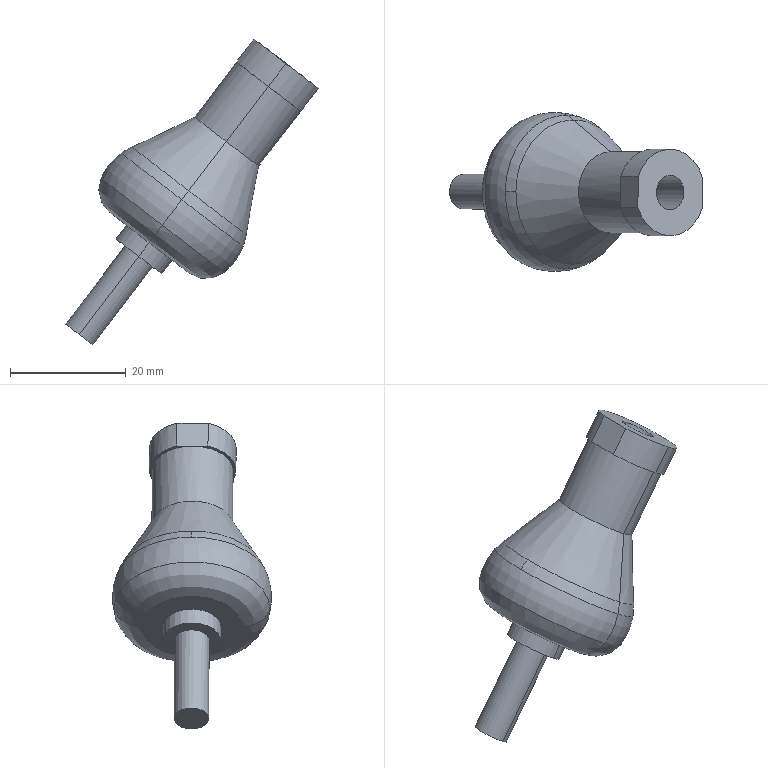Part | STEP file | 46B-01003ZX30 | 1 solid | 31 faces | box 43.778 x 27.592 x 52.956 mm | volume 12356 mm3 | cylinder 12 | plane 9 | torus 4 | sphere 4 | cone 2 | commonest cylinder face diameters 6 x4 15 x4 10 x2 14 x2
STEP:
#1=CARTESIAN_POINT('',(34.169,-36.791,43.691));
#2=VERTEX_POINT('',#1);
#3=CARTESIAN_POINT('',(34.207,-30.791,43.691));
#4=VERTEX_POINT('',#3);
#5=CARTESIAN_POINT('',(34.188,-33.791,43.691));
#6=DIRECTION('',(0.607,-0.003842,0.7947));
#7=AXIS2_PLACEMENT_3D('',#5,#6,$);
#8=CIRCLE('',#7,3.);
#9=EDGE_CURVE('',#2,#4,#8,.F.);
#10=ORIENTED_EDGE('',*,*,#9,.F.);
#11=CARTESIAN_POINT('',(44.488,-36.856,57.2));
#12=VERTEX_POINT('',#11);
#13=CARTESIAN_POINT('',(34.169,-36.791,43.691));
#14=DIRECTION('',(0.607,-0.003842,0.7947));
#15=VECTOR('',#14,1.);
#16=LINE('',#13,#15);
#17=EDGE_CURVE('',#2,#12,#16,.T.);
#18=ORIENTED_EDGE('',*,*,#17,.T.);
#19=CARTESIAN_POINT('',(44.526,-30.856,57.2));
#20=VERTEX_POINT('',#19);
#21=CARTESIAN_POINT('',(44.507,-33.856,57.2));
#22=DIRECTION('',(0.607,-0.003842,0.7947));
#23=AXIS2_PLACEMENT_3D('',#21,#22,$);
#24=CIRCLE('',#23,3.);
#25=EDGE_CURVE('',#12,#20,#24,.F.);
#26=ORIENTED_EDGE('',*,*,#25,.T.);
#27=CARTESIAN_POINT('',(34.207,-30.791,43.691));
#28=DIRECTION('',(0.607,-0.003842,0.7947));
#29=VECTOR('',#28,1.);
#30=LINE('',#27,#29);
#31=EDGE_CURVE('',#4,#20,#30,.T.);
#32=ORIENTED_EDGE('',*,*,#31,.F.);
#33=EDGE_LOOP('',(#10,#18,#26,#32));
#34=FACE_OUTER_BOUND('',#33,.T.);
#35=CARTESIAN_POINT('',(34.188,-33.791,43.691));
#36=DIRECTION('',(0.607,-0.003842,0.7947));
#37=DIRECTION('',(0.006329,1.,0.));
#38=AXIS2_PLACEMENT_3D('',#35,#36,#37);
#39=CYLINDRICAL_SURFACE('',#38,3.);
#40=ADVANCED_FACE('',(#34),#39,.T.);
#41=CARTESIAN_POINT('',(34.188,-33.791,43.691));
#42=DIRECTION('',(-0.607,0.003842,-0.7947));
#43=AXIS2_PLACEMENT_3D('',#41,#42,$);
#44=CIRCLE('',#43,3.);
#45=EDGE_CURVE('',#4,#2,#44,.T.);
#46=ORIENTED_EDGE('',*,*,#45,.T.);
#47=ORIENTED_EDGE('',*,*,#9,.T.);
#48=EDGE_LOOP('',(#46,#47));
#49=FACE_OUTER_BOUND('',#48,.T.);
#50=CARTESIAN_POINT('',(34.188,-33.791,43.691));
#51=DIRECTION('',(-0.607,0.003842,-0.7947));
#52=DIRECTION('',(-0.006329,-1.,0.));
#53=AXIS2_PLACEMENT_3D('',#50,#51,#52);
#54=PLANE('',#53);
#55=ADVANCED_FACE('',(#49),#54,.T.);
#56=ORIENTED_EDGE('',*,*,#17,.F.);
#57=ORIENTED_EDGE('',*,*,#45,.F.);
#58=ORIENTED_EDGE('',*,*,#31,.T.);
#59=CARTESIAN_POINT('',(44.507,-33.856,57.2));
#60=DIRECTION('',(0.607,-0.003842,0.7947));
#61=AXIS2_PLACEMENT_3D('',#59,#60,$);
#62=CIRCLE('',#61,3.);
#63=EDGE_CURVE('',#20,#12,#62,.F.);
#64=ORIENTED_EDGE('',*,*,#63,.T.);
#65=EDGE_LOOP('',(#56,#57,#58,#64));
#66=FACE_OUTER_BOUND('',#65,.T.);
#67=CARTESIAN_POINT('',(34.188,-33.791,43.691));
#68=DIRECTION('',(0.607,-0.003842,0.7947));
#69=DIRECTION('',(-0.006329,-1.,0.));
#70=AXIS2_PLACEMENT_3D('',#67,#68,#69);
#71=CYLINDRICAL_SURFACE('',#70,3.);
#72=ADVANCED_FACE('',(#66),#71,.T.);
#73=CARTESIAN_POINT('',(44.539,-28.857,57.2));
#74=VERTEX_POINT('',#73);
#75=CARTESIAN_POINT('',(44.476,-38.856,57.2));
#76=VERTEX_POINT('',#75);
#77=CARTESIAN_POINT('',(44.507,-33.856,57.2));
#78=DIRECTION('',(-0.607,0.003842,-0.7947));
#79=AXIS2_PLACEMENT_3D('',#77,#78,$);
#80=CIRCLE('',#79,5.);
#81=EDGE_CURVE('',#74,#76,#80,.T.);
#82=ORIENTED_EDGE('',*,*,#81,.T.);
#83=CARTESIAN_POINT('',(44.507,-33.856,57.2));
#84=DIRECTION('',(-0.607,0.003842,-0.7947));
#85=AXIS2_PLACEMENT_3D('',#83,#84,$);
#86=CIRCLE('',#85,5.);
#87=EDGE_CURVE('',#76,#74,#86,.T.);
#88=ORIENTED_EDGE('',*,*,#87,.T.);
#89=EDGE_LOOP('',(#82,#88));
#90=FACE_OUTER_BOUND('',#89,.T.);
#91=ORIENTED_EDGE('',*,*,#63,.F.);
#92=ORIENTED_EDGE('',*,*,#25,.F.);
#93=EDGE_LOOP('',(#91,#92));
#94=FACE_BOUND('',#93,.T.);
#95=CARTESIAN_POINT('',(44.507,-33.856,57.2));
#96=DIRECTION('',(-0.607,0.003842,-0.7947));
#97=DIRECTION('',(-0.006329,-1.,0.));
#98=AXIS2_PLACEMENT_3D('',#95,#96,#97);
#99=PLANE('',#98);
#100=ADVANCED_FACE('',(#90,#94),#99,.T.);
#101=CARTESIAN_POINT('',(46.297,-38.868,59.584));
#102=VERTEX_POINT('',#101);
#103=CARTESIAN_POINT('',(44.476,-38.856,57.2));
#104=DIRECTION('',(0.607,-0.003842,0.7947));
#105=VECTOR('',#104,1.);
#106=LINE('',#103,#105);
#107=EDGE_CURVE('',#76,#102,#106,.T.);
#108=ORIENTED_EDGE('',*,*,#107,.F.);
#109=ORIENTED_EDGE('',*,*,#81,.F.);
#110=CARTESIAN_POINT('',(46.36,-28.868,59.584));
#111=VERTEX_POINT('',#110);
#112=CARTESIAN_POINT('',(44.539,-28.857,57.2));
#113=DIRECTION('',(0.607,-0.003842,0.7947));
#114=VECTOR('',#113,1.);
#115=LINE('',#112,#114);
#116=EDGE_CURVE('',#74,#111,#115,.T.);
#117=ORIENTED_EDGE('',*,*,#116,.T.);
#118=CARTESIAN_POINT('',(46.328,-33.868,59.584));
#119=DIRECTION('',(0.607,-0.003842,0.7947));
#120=AXIS2_PLACEMENT_3D('',#118,#119,$);
#121=CIRCLE('',#120,5.);
#122=EDGE_CURVE('',#111,#102,#121,.F.);
#123=ORIENTED_EDGE('',*,*,#122,.T.);
#124=EDGE_LOOP('',(#108,#109,#117,#123));
#125=FACE_OUTER_BOUND('',#124,.T.);
#126=CARTESIAN_POINT('',(44.507,-33.856,57.2));
#127=DIRECTION('',(0.607,-0.003842,0.7947));
#128=DIRECTION('',(-0.006329,-1.,0.));
#129=AXIS2_PLACEMENT_3D('',#126,#127,#128);
#130=CYLINDRICAL_SURFACE('',#129,5.);
#131=ADVANCED_FACE('',(#125),#130,.T.);
#132=ORIENTED_EDGE('',*,*,#87,.F.);
#133=ORIENTED_EDGE('',*,*,#107,.T.);
#134=CARTESIAN_POINT('',(46.328,-33.868,59.584));
#135=DIRECTION('',(0.607,-0.003842,0.7947));
#136=AXIS2_PLACEMENT_3D('',#134,#135,$);
#137=CIRCLE('',#136,5.);
#138=EDGE_CURVE('',#102,#111,#137,.F.);
#139=ORIENTED_EDGE('',*,*,#138,.T.);
#140=ORIENTED_EDGE('',*,*,#116,.F.);
#141=EDGE_LOOP('',(#132,#133,#139,#140));
#142=FACE_OUTER_BOUND('',#141,.T.);
#143=CARTESIAN_POINT('',(44.507,-33.856,57.2));
#144=DIRECTION('',(0.607,-0.003842,0.7947));
#145=DIRECTION('',(0.006329,1.,0.));
#146=AXIS2_PLACEMENT_3D('',#143,#144,#145);
#147=CYLINDRICAL_SURFACE('',#146,5.);
#148=ADVANCED_FACE('',(#142),#147,.T.);
#149=CARTESIAN_POINT('',(46.274,-42.517,59.584));
#150=VERTEX_POINT('',#149);
#151=CARTESIAN_POINT('',(46.383,-25.219,59.584));
#152=VERTEX_POINT('',#151);
#153=CARTESIAN_POINT('',(46.328,-33.868,59.584));
#154=DIRECTION('',(-0.607,0.003842,-0.7947));
#155=AXIS2_PLACEMENT_3D('',#153,#154,$);
#156=CIRCLE('',#155,8.649);
#157=EDGE_CURVE('',#150,#152,#156,.T.);
#158=ORIENTED_EDGE('',*,*,#157,.T.);
#159=CARTESIAN_POINT('',(46.328,-33.868,59.584));
#160=DIRECTION('',(-0.607,0.003842,-0.7947));
#161=AXIS2_PLACEMENT_3D('',#159,#160,$);
#162=CIRCLE('',#161,8.649);
#163=EDGE_CURVE('',#152,#150,#162,.T.);
#164=ORIENTED_EDGE('',*,*,#163,.T.);
#165=EDGE_LOOP('',(#158,#164));
#166=FACE_OUTER_BOUND('',#165,.T.);
#167=ORIENTED_EDGE('',*,*,#122,.F.);
#168=ORIENTED_EDGE('',*,*,#138,.F.);
#169=EDGE_LOOP('',(#167,#168));
#170=FACE_BOUND('',#169,.T.);
#171=CARTESIAN_POINT('',(46.328,-33.868,59.584));
#172=DIRECTION('',(-0.607,0.003842,-0.7947));
#173=DIRECTION('',(-0.006329,-1.,0.));
#174=AXIS2_PLACEMENT_3D('',#171,#172,#173);
#175=PLANE('',#174);
#176=ADVANCED_FACE('',(#166,#170),#175,.T.);
#177=CARTESIAN_POINT('',(48.719,-20.38,62.602));
#178=VERTEX_POINT('',#177);
#179=CARTESIAN_POINT('',(48.548,-47.385,62.602));
#180=VERTEX_POINT('',#179);
#181=CARTESIAN_POINT('',(48.633,-33.883,62.602));
#182=DIRECTION('',(-0.607,0.003842,-0.7947));
#183=AXIS2_PLACEMENT_3D('',#181,#182,$);
#184=CIRCLE('',#183,13.502);
#185=EDGE_CURVE('',#178,#180,#184,.F.);
#186=ORIENTED_EDGE('',*,*,#185,.F.);
#187=CARTESIAN_POINT('',(49.418,-25.238,63.558));
#188=DIRECTION('',(-0.7947,0.00503,0.607));
#189=AXIS2_PLACEMENT_3D('',#187,#188,$);
#190=CIRCLE('',#189,5.);
#191=EDGE_CURVE('',#178,#152,#190,.T.);
#192=ORIENTED_EDGE('',*,*,#191,.T.);
#193=ORIENTED_EDGE('',*,*,#157,.F.);
#194=CARTESIAN_POINT('',(49.309,-42.536,63.558));
#195=DIRECTION('',(0.7947,-0.00503,-0.607));
#196=AXIS2_PLACEMENT_3D('',#194,#195,$);
#197=CIRCLE('',#196,5.);
#198=EDGE_CURVE('',#180,#150,#197,.T.);
#199=ORIENTED_EDGE('',*,*,#198,.F.);
#200=EDGE_LOOP('',(#186,#192,#193,#199));
#201=FACE_OUTER_BOUND('',#200,.T.);
#202=CARTESIAN_POINT('',(49.364,-33.887,63.558));
#203=DIRECTION('',(-0.607,0.003842,-0.7947));
#204=DIRECTION('',(-0.006329,-1.,0.));
#205=AXIS2_PLACEMENT_3D('',#202,#203,#204);
#206=TOROIDAL_SURFACE('',#205,8.649,5.);
#207=ADVANCED_FACE('',(#201),#206,.T.);
#208=ORIENTED_EDGE('',*,*,#191,.F.);
#209=CARTESIAN_POINT('',(48.633,-33.883,62.602));
#210=DIRECTION('',(-0.607,0.003842,-0.7947));
#211=AXIS2_PLACEMENT_3D('',#209,#210,$);
#212=CIRCLE('',#211,13.502);
#213=EDGE_CURVE('',#180,#178,#212,.F.);
#214=ORIENTED_EDGE('',*,*,#213,.F.);
#215=ORIENTED_EDGE('',*,*,#198,.T.);
#216=ORIENTED_EDGE('',*,*,#163,.F.);
#217=EDGE_LOOP('',(#208,#214,#215,#216));
#218=FACE_OUTER_BOUND('',#217,.T.);
#219=CARTESIAN_POINT('',(49.364,-33.887,63.558));
#220=DIRECTION('',(-0.607,0.003842,-0.7947));
#221=DIRECTION('',(0.006329,1.,0.));
#222=AXIS2_PLACEMENT_3D('',#219,#220,#221);
#223=TOROIDAL_SURFACE('',#222,8.649,5.);
#224=ADVANCED_FACE('',(#218),#223,.T.);
#225=CARTESIAN_POINT('',(52.092,-20.618,67.019));
#226=VERTEX_POINT('',#225);
#227=CARTESIAN_POINT('',(41.45,-33.837,75.084));
#228=VERTEX_POINT('',#227);
#229=CARTESIAN_POINT('',(52.008,-33.904,67.019));
#230=DIRECTION('',(-0.607,0.003842,-0.7947));
#231=AXIS2_PLACEMENT_3D('',#229,#230,$);
#232=CIRCLE('',#231,13.286);
#233=EDGE_CURVE('',#226,#228,#232,.F.);
#234=ORIENTED_EDGE('',*,*,#233,.F.);
#235=CARTESIAN_POINT('',(50.118,-30.096,64.513));
#236=DIRECTION('',(-0.7947,0.00503,0.607));
#237=AXIS2_PLACEMENT_3D('',#235,#236,$);
#238=CIRCLE('',#237,10.);
#239=EDGE_CURVE('',#226,#178,#238,.T.);
#240=ORIENTED_EDGE('',*,*,#239,.T.);
#241=ORIENTED_EDGE('',*,*,#185,.T.);
#242=CARTESIAN_POINT('',(51.924,-47.189,67.019));
#243=VERTEX_POINT('',#242);
#244=CARTESIAN_POINT('',(50.069,-37.688,64.513));
#245=DIRECTION('',(0.7947,-0.00503,-0.607));
#246=AXIS2_PLACEMENT_3D('',#244,#245,$);
#247=CIRCLE('',#246,10.);
#248=EDGE_CURVE('',#243,#180,#247,.T.);
#249=ORIENTED_EDGE('',*,*,#248,.F.);
#250=CARTESIAN_POINT('',(52.008,-33.904,67.019));
#251=DIRECTION('',(-0.607,0.003842,-0.7947));
#252=AXIS2_PLACEMENT_3D('',#250,#251,$);
#253=CIRCLE('',#252,13.286);
#254=EDGE_CURVE('',#228,#243,#253,.F.);
#255=ORIENTED_EDGE('',*,*,#254,.F.);
#256=EDGE_LOOP('',(#234,#240,#241,#249,#255));
#257=FACE_OUTER_BOUND('',#256,.T.);
#258=CARTESIAN_POINT('',(50.094,-33.892,64.513));
#259=DIRECTION('',(-0.607,0.003842,-0.7947));
#260=DIRECTION('',(-0.006329,-1.,0.));
#261=AXIS2_PLACEMENT_3D('',#258,#259,#260);
#262=DEGENERATE_TOROIDAL_SURFACE('',#261,3.796,10.,.T.);
#263=ADVANCED_FACE('',(#257),#262,.T.);
#264=ORIENTED_EDGE('',*,*,#239,.F.);
#265=CARTESIAN_POINT('',(62.565,-33.971,58.954));
#266=VERTEX_POINT('',#265);
#267=CARTESIAN_POINT('',(52.008,-33.904,67.019));
#268=DIRECTION('',(-0.607,0.003842,-0.7947));
#269=AXIS2_PLACEMENT_3D('',#267,#268,$);
#270=CIRCLE('',#269,13.286);
#271=EDGE_CURVE('',#266,#226,#270,.F.);
#272=ORIENTED_EDGE('',*,*,#271,.F.);
#273=CARTESIAN_POINT('',(52.008,-33.904,67.019));
#274=DIRECTION('',(-0.607,0.003842,-0.7947));
#275=AXIS2_PLACEMENT_3D('',#273,#274,$);
#276=CIRCLE('',#275,13.286);
#277=EDGE_CURVE('',#243,#266,#276,.F.);
#278=ORIENTED_EDGE('',*,*,#277,.F.);
#279=ORIENTED_EDGE('',*,*,#248,.T.);
#280=ORIENTED_EDGE('',*,*,#213,.T.);
#281=EDGE_LOOP('',(#264,#272,#278,#279,#280));
#282=FACE_OUTER_BOUND('',#281,.T.);
#283=CARTESIAN_POINT('',(50.094,-33.892,64.513));
#284=DIRECTION('',(-0.607,0.003842,-0.7947));
#285=DIRECTION('',(0.006329,1.,0.));
#286=AXIS2_PLACEMENT_3D('',#283,#284,#285);
#287=DEGENERATE_TOROIDAL_SURFACE('',#286,3.796,10.,.T.);
#288=ADVANCED_FACE('',(#282),#287,.T.);
#289=CARTESIAN_POINT('',(53.277,-21.447,68.577));
#290=VERTEX_POINT('',#289);
#291=CARTESIAN_POINT('',(49.328,-33.887,63.511));
#292=DIRECTION('',(0.7947,-0.00503,-0.607));
#293=AXIS2_PLACEMENT_3D('',#291,#292,$);
#294=CIRCLE('',#293,14.);
#295=EDGE_CURVE('',#226,#290,#294,.T.);
#296=ORIENTED_EDGE('',*,*,#295,.F.);
#297=ORIENTED_EDGE('',*,*,#233,.T.);
#298=CARTESIAN_POINT('',(43.293,-33.849,76.143));
#299=VERTEX_POINT('',#298);
#300=CARTESIAN_POINT('',(49.328,-33.887,63.511));
#301=DIRECTION('',(-0.006329,-1.,0.));
#302=AXIS2_PLACEMENT_3D('',#300,#301,$);
#303=CIRCLE('',#302,14.);
#304=EDGE_CURVE('',#228,#299,#303,.F.);
#305=ORIENTED_EDGE('',*,*,#304,.T.);
#306=CARTESIAN_POINT('',(53.277,-21.447,68.577));
#307=CARTESIAN_POINT('',(52.881,-21.445,68.879));
#308=CARTESIAN_POINT('',(52.485,-21.467,69.181));
#309=CARTESIAN_POINT('',(52.082,-21.514,69.489));
#310=CARTESIAN_POINT('',(51.216,-21.672,70.15));
#311=CARTESIAN_POINT('',(50.266,-21.99,70.874));
#312=CARTESIAN_POINT('',(49.746,-22.207,71.27));
#313=CARTESIAN_POINT('',(48.645,-22.788,72.108));
#314=CARTESIAN_POINT('',(47.509,-23.675,72.972));
#315=CARTESIAN_POINT('',(46.946,-24.205,73.399));
#316=CARTESIAN_POINT('',(45.885,-25.41,74.204));
#317=CARTESIAN_POINT('',(44.991,-26.871,74.88));
#318=CARTESIAN_POINT('',(44.598,-27.656,75.176));
#319=CARTESIAN_POINT('',(43.93,-29.311,75.679));
#320=CARTESIAN_POINT('',(43.513,-31.094,75.988));
#321=CARTESIAN_POINT('',(43.372,-32.005,76.091));
#322=CARTESIAN_POINT('',(43.299,-32.927,76.143));
#323=CARTESIAN_POINT('',(43.293,-33.849,76.143));
#324=B_SPLINE_CURVE_WITH_KNOTS('',5,(#306,#307,#308,#309,#310,#311,#312,#313,#314,#315,#316,#317,#318,#319,#320,#321,#322,#323),.UNSPECIFIED.,.F.,.U.,(6,3,3,3,3,6),(0.,6.005,12.466,19.014,25.534,32.054),.UNSPECIFIED.);
#325=EDGE_CURVE('',#290,#299,#324,.T.);
#326=ORIENTED_EDGE('',*,*,#325,.F.);
#327=EDGE_LOOP('',(#296,#297,#305,#326));
#328=FACE_OUTER_BOUND('',#327,.T.);
#329=CARTESIAN_POINT('',(49.328,-33.887,63.511));
#330=DIRECTION('',(-0.006329,-1.,0.));
#331=DIRECTION('',(0.607,-0.003842,0.7947));
#332=AXIS2_PLACEMENT_3D('',#329,#330,#331);
#333=SPHERICAL_SURFACE('',#332,14.);
#334=ADVANCED_FACE('',(#328),#333,.T.);
#335=CARTESIAN_POINT('',(53.119,-46.375,68.577));
#336=VERTEX_POINT('',#335);
#337=CARTESIAN_POINT('',(49.328,-33.887,63.511));
#338=DIRECTION('',(0.7947,-0.00503,-0.607));
#339=AXIS2_PLACEMENT_3D('',#337,#338,$);
#340=CIRCLE('',#339,14.);
#341=EDGE_CURVE('',#336,#243,#340,.T.);
#342=ORIENTED_EDGE('',*,*,#341,.F.);
#343=CARTESIAN_POINT('',(43.293,-33.849,76.143));
#344=CARTESIAN_POINT('',(43.281,-35.755,76.143));
#345=CARTESIAN_POINT('',(43.558,-37.662,75.922));
#346=CARTESIAN_POINT('',(44.129,-39.501,75.477));
#347=CARTESIAN_POINT('',(45.385,-41.93,74.506));
#348=CARTESIAN_POINT('',(47.022,-43.742,73.247));
#349=CARTESIAN_POINT('',(47.59,-44.26,72.81));
#350=CARTESIAN_POINT('',(48.736,-45.126,71.931));
#351=CARTESIAN_POINT('',(49.833,-45.681,71.09));
#352=CARTESIAN_POINT('',(50.354,-45.888,70.691));
#353=CARTESIAN_POINT('',(51.241,-46.168,70.012));
#354=CARTESIAN_POINT('',(52.061,-46.31,69.386));
#355=CARTESIAN_POINT('',(52.417,-46.351,69.113));
#356=CARTESIAN_POINT('',(52.768,-46.373,68.845));
#357=CARTESIAN_POINT('',(53.119,-46.375,68.577));
#358=B_SPLINE_CURVE_WITH_KNOTS('',5,(#343,#344,#345,#346,#347,#348,#349,#350,#351,#352,#353,#354,#355,#356,#357),.UNSPECIFIED.,.F.,.U.,(6,3,3,3,6),(0.,13.477,20.093,26.711,32.042),.UNSPECIFIED.);
#359=EDGE_CURVE('',#299,#336,#358,.T.);
#360=ORIENTED_EDGE('',*,*,#359,.F.);
#361=ORIENTED_EDGE('',*,*,#304,.F.);
#362=ORIENTED_EDGE('',*,*,#254,.T.);
#363=EDGE_LOOP('',(#342,#360,#361,#362));
#364=FACE_OUTER_BOUND('',#363,.T.);
#365=CARTESIAN_POINT('',(49.328,-33.887,63.511));
#366=DIRECTION('',(-0.006329,-1.,0.));
#367=DIRECTION('',(0.607,-0.003842,0.7947));
#368=AXIS2_PLACEMENT_3D('',#365,#366,#367);
#369=SPHERICAL_SURFACE('',#368,14.);
#370=ADVANCED_FACE('',(#364),#369,.T.);
#371=ORIENTED_EDGE('',*,*,#295,.T.);
#372=CARTESIAN_POINT('',(63.103,-33.974,61.011));
#373=VERTEX_POINT('',#372);
#374=CARTESIAN_POINT('',(63.103,-33.974,61.011));
#375=CARTESIAN_POINT('',(63.115,-32.068,61.011));
#376=CARTESIAN_POINT('',(62.837,-30.16,61.232));
#377=CARTESIAN_POINT('',(62.266,-28.322,61.677));
#378=CARTESIAN_POINT('',(61.01,-25.893,62.648));
#379=CARTESIAN_POINT('',(59.373,-24.081,63.907));
#380=CARTESIAN_POINT('',(58.805,-23.563,64.343));
#381=CARTESIAN_POINT('',(57.659,-22.697,65.223));
#382=CARTESIAN_POINT('',(56.562,-22.142,66.064));
#383=CARTESIAN_POINT('',(56.042,-21.935,66.462));
#384=CARTESIAN_POINT('',(55.154,-21.655,67.142));
#385=CARTESIAN_POINT('',(54.335,-21.513,67.768));
#386=CARTESIAN_POINT('',(53.979,-21.471,68.04));
#387=CARTESIAN_POINT('',(53.628,-21.45,68.309));
#388=CARTESIAN_POINT('',(53.277,-21.447,68.577));
#389=B_SPLINE_CURVE_WITH_KNOTS('',5,(#374,#375,#376,#377,#378,#379,#380,#381,#382,#383,#384,#385,#386,#387,#388),.UNSPECIFIED.,.F.,.U.,(6,3,3,3,6),(0.,13.477,20.093,26.711,32.042),.UNSPECIFIED.);
#390=EDGE_CURVE('',#373,#290,#389,.T.);
#391=ORIENTED_EDGE('',*,*,#390,.F.);
#392=CARTESIAN_POINT('',(49.328,-33.887,63.511));
#393=DIRECTION('',(-0.006329,-1.,0.));
#394=AXIS2_PLACEMENT_3D('',#392,#393,$);
#395=CIRCLE('',#394,14.);
#396=EDGE_CURVE('',#266,#373,#395,.T.);
#397=ORIENTED_EDGE('',*,*,#396,.F.);
#398=ORIENTED_EDGE('',*,*,#271,.T.);
#399=EDGE_LOOP('',(#371,#391,#397,#398));
#400=FACE_OUTER_BOUND('',#399,.T.);
#401=CARTESIAN_POINT('',(49.328,-33.887,63.511));
#402=DIRECTION('',(-0.006329,-1.,0.));
#403=DIRECTION('',(0.7947,-0.00503,-0.607));
#404=AXIS2_PLACEMENT_3D('',#401,#402,#403);
#405=SPHERICAL_SURFACE('',#404,14.);
#406=ADVANCED_FACE('',(#400),#405,.T.);
#407=ORIENTED_EDGE('',*,*,#341,.T.);
#408=ORIENTED_EDGE('',*,*,#277,.T.);
#409=ORIENTED_EDGE('',*,*,#396,.T.);
#410=CARTESIAN_POINT('',(53.119,-46.375,68.577));
#411=CARTESIAN_POINT('',(53.514,-46.378,68.275));
#412=CARTESIAN_POINT('',(53.91,-46.356,67.973));
#413=CARTESIAN_POINT('',(54.313,-46.308,67.665));
#414=CARTESIAN_POINT('',(55.18,-46.151,67.004));
#415=CARTESIAN_POINT('',(56.129,-45.833,66.28));
#416=CARTESIAN_POINT('',(56.649,-45.616,65.884));
#417=CARTESIAN_POINT('',(57.75,-45.035,65.046));
#418=CARTESIAN_POINT('',(58.886,-44.148,64.182));
#419=CARTESIAN_POINT('',(59.449,-43.618,63.754));
#420=CARTESIAN_POINT('',(60.511,-42.413,62.95));
#421=CARTESIAN_POINT('',(61.404,-40.952,62.274));
#422=CARTESIAN_POINT('',(61.798,-40.167,61.977));
#423=CARTESIAN_POINT('',(62.466,-38.512,61.475));
#424=CARTESIAN_POINT('',(62.882,-36.729,61.166));
#425=CARTESIAN_POINT('',(63.023,-35.818,61.062));
#426=CARTESIAN_POINT('',(63.097,-34.896,61.011));
#427=CARTESIAN_POINT('',(63.103,-33.974,61.011));
#428=B_SPLINE_CURVE_WITH_KNOTS('',5,(#410,#411,#412,#413,#414,#415,#416,#417,#418,#419,#420,#421,#422,#423,#424,#425,#426,#427),.UNSPECIFIED.,.F.,.U.,(6,3,3,3,3,6),(0.,6.005,12.466,19.014,25.534,32.054),.UNSPECIFIED.);
#429=EDGE_CURVE('',#336,#373,#428,.T.);
#430=ORIENTED_EDGE('',*,*,#429,.F.);
#431=EDGE_LOOP('',(#407,#408,#409,#430));
#432=FACE_OUTER_BOUND('',#431,.T.);
#433=CARTESIAN_POINT('',(49.328,-33.887,63.511));
#434=DIRECTION('',(-0.006329,-1.,0.));
#435=DIRECTION('',(0.7947,-0.00503,-0.607));
#436=AXIS2_PLACEMENT_3D('',#433,#434,#435);
#437=SPHERICAL_SURFACE('',#436,14.);
#438=ADVANCED_FACE('',(#432),#437,.T.);
#439=CARTESIAN_POINT('',(59.727,-26.953,77.067));
#440=VERTEX_POINT('',#439);
#441=CARTESIAN_POINT('',(59.639,-40.952,77.067));
#442=VERTEX_POINT('',#441);
#443=CARTESIAN_POINT('',(59.683,-33.952,77.067));
#444=DIRECTION('',(-0.607,0.003842,-0.7947));
#445=AXIS2_PLACEMENT_3D('',#443,#444,$);
#446=CIRCLE('',#445,7.);
#447=EDGE_CURVE('',#440,#442,#446,.F.);
#448=ORIENTED_EDGE('',*,*,#447,.F.);
#449=CARTESIAN_POINT('',(-268715.502,229354.82,-353668.877));
#450=DIRECTION('',(-0.5376,0.4588,-0.7075));
#451=VECTOR('',#450,1.);
#452=LINE('',#449,#451);
#453=EDGE_CURVE('',#440,#290,#452,.T.);
#454=ORIENTED_EDGE('',*,*,#453,.T.);
#455=ORIENTED_EDGE('',*,*,#325,.T.);
#456=ORIENTED_EDGE('',*,*,#359,.T.);
#457=CARTESIAN_POINT('',(-271597.559,-226002.206,-353668.877));
#458=DIRECTION('',(-0.5433,-0.4519,-0.7075));
#459=VECTOR('',#458,1.);
#460=LINE('',#457,#459);
#461=EDGE_CURVE('',#442,#336,#460,.T.);
#462=ORIENTED_EDGE('',*,*,#461,.F.);
#463=EDGE_LOOP('',(#448,#454,#455,#456,#462));
#464=FACE_OUTER_BOUND('',#463,.T.);
#465=CARTESIAN_POINT('',(59.683,-33.952,77.067));
#466=DIRECTION('',(-0.607,0.003842,-0.7947));
#467=DIRECTION('',(-0.006329,-1.,0.));
#468=AXIS2_PLACEMENT_3D('',#465,#466,#467);
#469=CONICAL_SURFACE('',#468,7.,0.4728);
#470=ADVANCED_FACE('',(#464),#469,.T.);
#471=ORIENTED_EDGE('',*,*,#453,.F.);
#472=CARTESIAN_POINT('',(59.683,-33.952,77.067));
#473=DIRECTION('',(-0.607,0.003842,-0.7947));
#474=AXIS2_PLACEMENT_3D('',#472,#473,$);
#475=CIRCLE('',#474,7.);
#476=EDGE_CURVE('',#442,#440,#475,.F.);
#477=ORIENTED_EDGE('',*,*,#476,.F.);
#478=ORIENTED_EDGE('',*,*,#461,.T.);
#479=ORIENTED_EDGE('',*,*,#429,.T.);
#480=ORIENTED_EDGE('',*,*,#390,.T.);
#481=EDGE_LOOP('',(#471,#477,#478,#479,#480));
#482=FACE_OUTER_BOUND('',#481,.T.);
#483=CARTESIAN_POINT('',(59.683,-33.952,77.067));
#484=DIRECTION('',(-0.607,0.003842,-0.7947));
#485=DIRECTION('',(0.006329,1.,0.));
#486=AXIS2_PLACEMENT_3D('',#483,#484,#485);
#487=CONICAL_SURFACE('',#486,7.,0.4728);
#488=ADVANCED_FACE('',(#482),#487,.T.);
#489=ORIENTED_EDGE('',*,*,#447,.T.);
#490=CARTESIAN_POINT('',(66.923,-40.998,86.603));
#491=VERTEX_POINT('',#490);
#492=CARTESIAN_POINT('',(69.958,-41.018,90.576));
#493=DIRECTION('',(0.607,-0.003842,0.7947));
#494=VECTOR('',#493,1.);
#495=LINE('',#492,#494);
#496=EDGE_CURVE('',#442,#491,#495,.T.);
#497=ORIENTED_EDGE('',*,*,#496,.T.);
#498=CARTESIAN_POINT('',(61.405,-33.963,90.852));
#499=VERTEX_POINT('',#498);
#500=CARTESIAN_POINT('',(66.967,-33.999,86.603));
#501=DIRECTION('',(0.607,-0.003842,0.7947));
#502=AXIS2_PLACEMENT_3D('',#500,#501,$);
#503=CIRCLE('',#502,7.);
#504=EDGE_CURVE('',#499,#491,#503,.T.);
#505=ORIENTED_EDGE('',*,*,#504,.F.);
#506=CARTESIAN_POINT('',(67.012,-26.999,86.603));
#507=VERTEX_POINT('',#506);
#508=CARTESIAN_POINT('',(66.967,-33.999,86.603));
#509=DIRECTION('',(0.607,-0.003842,0.7947));
#510=AXIS2_PLACEMENT_3D('',#508,#509,$);
#511=CIRCLE('',#510,7.);
#512=EDGE_CURVE('',#507,#499,#511,.T.);
#513=ORIENTED_EDGE('',*,*,#512,.F.);
#514=CARTESIAN_POINT('',(70.047,-27.018,90.576));
#515=DIRECTION('',(0.607,-0.003842,0.7947));
#516=VECTOR('',#515,1.);
#517=LINE('',#514,#516);
#518=EDGE_CURVE('',#440,#507,#517,.T.);
#519=ORIENTED_EDGE('',*,*,#518,.F.);
#520=EDGE_LOOP('',(#489,#497,#505,#513,#519));
#521=FACE_OUTER_BOUND('',#520,.T.);
#522=CARTESIAN_POINT('',(70.002,-34.018,90.576));
#523=DIRECTION('',(0.607,-0.003842,0.7947));
#524=DIRECTION('',(0.006329,1.,0.));
#525=AXIS2_PLACEMENT_3D('',#522,#523,#524);
#526=CYLINDRICAL_SURFACE('',#525,7.);
#527=ADVANCED_FACE('',(#521),#526,.T.);
#528=ORIENTED_EDGE('',*,*,#496,.F.);
#529=ORIENTED_EDGE('',*,*,#476,.T.);
#530=ORIENTED_EDGE('',*,*,#518,.T.);
#531=CARTESIAN_POINT('',(72.53,-34.034,82.354));
#532=VERTEX_POINT('',#531);
#533=CARTESIAN_POINT('',(66.967,-33.999,86.603));
#534=DIRECTION('',(0.607,-0.003842,0.7947));
#535=AXIS2_PLACEMENT_3D('',#533,#534,$);
#536=CIRCLE('',#535,7.);
#537=EDGE_CURVE('',#532,#507,#536,.T.);
#538=ORIENTED_EDGE('',*,*,#537,.F.);
#539=CARTESIAN_POINT('',(66.967,-33.999,86.603));
#540=DIRECTION('',(0.607,-0.003842,0.7947));
#541=AXIS2_PLACEMENT_3D('',#539,#540,$);
#542=CIRCLE('',#541,7.);
#543=EDGE_CURVE('',#491,#532,#542,.T.);
#544=ORIENTED_EDGE('',*,*,#543,.F.);
#545=EDGE_LOOP('',(#528,#529,#530,#538,#544));
#546=FACE_OUTER_BOUND('',#545,.T.);
#547=CARTESIAN_POINT('',(70.002,-34.018,90.576));
#548=DIRECTION('',(0.607,-0.003842,0.7947));
#549=DIRECTION('',(-0.006329,-1.,0.));
#550=AXIS2_PLACEMENT_3D('',#547,#548,#549);
#551=CYLINDRICAL_SURFACE('',#550,7.);
#552=ADVANCED_FACE('',(#546),#551,.T.);
#553=CARTESIAN_POINT('',(61.388,-36.656,90.852));
#554=VERTEX_POINT('',#553);
#555=CARTESIAN_POINT('',(61.396,-35.31,90.852));
#556=DIRECTION('',(0.006329,1.,0.));
#557=VECTOR('',#556,1.);
#558=LINE('',#555,#557);
#559=EDGE_CURVE('',#554,#499,#558,.T.);
#560=ORIENTED_EDGE('',*,*,#559,.T.);
#561=ORIENTED_EDGE('',*,*,#504,.T.);
#562=ORIENTED_EDGE('',*,*,#543,.T.);
#563=CARTESIAN_POINT('',(72.513,-36.726,82.354));
#564=VERTEX_POINT('',#563);
#565=CARTESIAN_POINT('',(72.521,-35.38,82.354));
#566=DIRECTION('',(-0.006329,-1.,0.));
#567=VECTOR('',#566,1.);
#568=LINE('',#565,#567);
#569=EDGE_CURVE('',#532,#564,#568,.T.);
#570=ORIENTED_EDGE('',*,*,#569,.T.);
#571=CARTESIAN_POINT('',(66.92,-41.498,86.603));
#572=VERTEX_POINT('',#571);
#573=CARTESIAN_POINT('',(66.92,-41.498,86.603));
#574=CARTESIAN_POINT('',(67.404,-41.501,86.233));
#575=CARTESIAN_POINT('',(67.889,-41.443,85.863));
#576=CARTESIAN_POINT('',(68.368,-41.322,85.498));
#577=CARTESIAN_POINT('',(69.448,-40.901,84.675));
#578=CARTESIAN_POINT('',(70.425,-40.174,83.932));
#579=CARTESIAN_POINT('',(70.934,-39.668,83.545));
#580=CARTESIAN_POINT('',(71.601,-38.799,83.04));
#581=CARTESIAN_POINT('',(72.116,-37.789,82.652));
#582=CARTESIAN_POINT('',(72.266,-37.445,82.538));
#583=CARTESIAN_POINT('',(72.399,-37.09,82.439));
#584=CARTESIAN_POINT('',(72.513,-36.726,82.354));
#585=B_SPLINE_CURVE_WITH_KNOTS('',5,(#573,#574,#575,#576,#577,#578,#579,#580,#581,#582,#583,#584),.UNSPECIFIED.,.F.,.U.,(6,3,3,6),(12.766,17.076,22.768,25.532),.UNSPECIFIED.);
#586=EDGE_CURVE('',#572,#564,#585,.T.);
#587=ORIENTED_EDGE('',*,*,#586,.F.);
#588=CARTESIAN_POINT('',(61.388,-36.656,90.852));
#589=CARTESIAN_POINT('',(61.613,-37.409,90.677));
#590=CARTESIAN_POINT('',(61.918,-38.123,90.44));
#591=CARTESIAN_POINT('',(62.298,-38.781,90.147));
#592=CARTESIAN_POINT('',(63.19,-39.953,89.46));
#593=CARTESIAN_POINT('',(64.296,-40.786,88.611));
#594=CARTESIAN_POINT('',(64.891,-41.106,88.155));
#595=CARTESIAN_POINT('',(65.663,-41.374,87.563));
#596=CARTESIAN_POINT('',(66.454,-41.476,86.959));
#597=CARTESIAN_POINT('',(66.609,-41.49,86.84));
#598=CARTESIAN_POINT('',(66.765,-41.497,86.722));
#599=CARTESIAN_POINT('',(66.92,-41.498,86.603));
#600=B_SPLINE_CURVE_WITH_KNOTS('',5,(#588,#589,#590,#591,#592,#593,#594,#595,#596,#597,#598,#599),.UNSPECIFIED.,.F.,.U.,(6,3,3,6),(0.,5.692,11.384,12.766),.UNSPECIFIED.);
#601=EDGE_CURVE('',#554,#572,#600,.T.);
#602=ORIENTED_EDGE('',*,*,#601,.F.);
#603=EDGE_LOOP('',(#560,#561,#562,#570,#587,#602));
#604=FACE_OUTER_BOUND('',#603,.T.);
#605=CARTESIAN_POINT('',(61.007,-33.961,91.156));
#606=DIRECTION('',(-0.607,0.003842,-0.7947));
#607=DIRECTION('',(-0.006329,-1.,0.));
#608=AXIS2_PLACEMENT_3D('',#605,#606,#607);
#609=PLANE('',#608);
#610=ADVANCED_FACE('',(#604),#609,.T.);
#611=CARTESIAN_POINT('',(61.422,-31.271,90.852));
#612=VERTEX_POINT('',#611);
#613=CARTESIAN_POINT('',(61.413,-32.617,90.852));
#614=DIRECTION('',(0.006329,1.,0.));
#615=VECTOR('',#614,1.);
#616=LINE('',#613,#615);
#617=EDGE_CURVE('',#499,#612,#616,.T.);
#618=ORIENTED_EDGE('',*,*,#617,.T.);
#619=CARTESIAN_POINT('',(67.015,-26.499,86.603));
#620=VERTEX_POINT('',#619);
#621=CARTESIAN_POINT('',(67.015,-26.499,86.603));
#622=CARTESIAN_POINT('',(66.375,-26.495,87.092));
#623=CARTESIAN_POINT('',(65.735,-26.599,87.58));
#624=CARTESIAN_POINT('',(65.109,-26.811,88.057));
#625=CARTESIAN_POINT('',(63.918,-27.441,88.964));
#626=CARTESIAN_POINT('',(62.9,-28.443,89.737));
#627=CARTESIAN_POINT('',(62.447,-29.027,90.08));
#628=CARTESIAN_POINT('',(61.969,-29.84,90.441));
#629=CARTESIAN_POINT('',(61.607,-30.732,90.714));
#630=CARTESIAN_POINT('',(61.54,-30.909,90.764));
#631=CARTESIAN_POINT('',(61.479,-31.089,90.81));
#632=CARTESIAN_POINT('',(61.422,-31.271,90.852));
#633=B_SPLINE_CURVE_WITH_KNOTS('',5,(#621,#622,#623,#624,#625,#626,#627,#628,#629,#630,#631,#632),.UNSPECIFIED.,.F.,.U.,(6,3,3,6),(0.,5.692,11.384,12.765),.UNSPECIFIED.);
#634=EDGE_CURVE('',#620,#612,#633,.T.);
#635=ORIENTED_EDGE('',*,*,#634,.F.);
#636=CARTESIAN_POINT('',(72.547,-31.341,82.354));
#637=VERTEX_POINT('',#636);
#638=CARTESIAN_POINT('',(72.547,-31.341,82.354));
#639=CARTESIAN_POINT('',(72.322,-30.589,82.529));
#640=CARTESIAN_POINT('',(72.017,-29.874,82.766));
#641=CARTESIAN_POINT('',(71.637,-29.216,83.059));
#642=CARTESIAN_POINT('',(70.745,-28.045,83.746));
#643=CARTESIAN_POINT('',(69.639,-27.211,84.595));
#644=CARTESIAN_POINT('',(69.044,-26.891,85.051));
#645=CARTESIAN_POINT('',(68.271,-26.623,85.643));
#646=CARTESIAN_POINT('',(67.48,-26.521,86.247));
#647=CARTESIAN_POINT('',(67.325,-26.507,86.366));
#648=CARTESIAN_POINT('',(67.17,-26.5,86.484));
#649=CARTESIAN_POINT('',(67.015,-26.499,86.603));
#650=B_SPLINE_CURVE_WITH_KNOTS('',5,(#638,#639,#640,#641,#642,#643,#644,#645,#646,#647,#648,#649),.UNSPECIFIED.,.F.,.U.,(6,3,3,6),(0.,5.692,11.384,12.765),.UNSPECIFIED.);
#651=EDGE_CURVE('',#637,#620,#650,.T.);
#652=ORIENTED_EDGE('',*,*,#651,.F.);
#653=CARTESIAN_POINT('',(72.538,-32.688,82.354));
#654=DIRECTION('',(-0.006329,-1.,0.));
#655=VECTOR('',#654,1.);
#656=LINE('',#653,#655);
#657=EDGE_CURVE('',#637,#532,#656,.T.);
#658=ORIENTED_EDGE('',*,*,#657,.T.);
#659=ORIENTED_EDGE('',*,*,#537,.T.);
#660=ORIENTED_EDGE('',*,*,#512,.T.);
#661=EDGE_LOOP('',(#618,#635,#652,#658,#659,#660));
#662=FACE_OUTER_BOUND('',#661,.T.);
#663=CARTESIAN_POINT('',(61.007,-33.961,91.156));
#664=DIRECTION('',(-0.607,0.003842,-0.7947));
#665=DIRECTION('',(-0.006329,-1.,0.));
#666=AXIS2_PLACEMENT_3D('',#663,#664,#665);
#667=PLANE('',#666);
#668=ADVANCED_FACE('',(#662),#667,.T.);
#669=CARTESIAN_POINT('',(64.457,-31.29,94.826));
#670=VERTEX_POINT('',#669);
#671=CARTESIAN_POINT('',(62.939,-31.28,92.839));
#672=DIRECTION('',(-0.607,0.003842,-0.7947));
#673=VECTOR('',#672,1.);
#674=LINE('',#671,#673);
#675=EDGE_CURVE('',#670,#612,#674,.T.);
#676=ORIENTED_EDGE('',*,*,#675,.T.);
#677=ORIENTED_EDGE('',*,*,#617,.F.);
#678=ORIENTED_EDGE('',*,*,#559,.F.);
#679=CARTESIAN_POINT('',(64.423,-36.675,94.826));
#680=VERTEX_POINT('',#679);
#681=CARTESIAN_POINT('',(62.905,-36.666,92.839));
#682=DIRECTION('',(0.607,-0.003842,0.7947));
#683=VECTOR('',#682,1.);
#684=LINE('',#681,#683);
#685=EDGE_CURVE('',#554,#680,#684,.T.);
#686=ORIENTED_EDGE('',*,*,#685,.T.);
#687=CARTESIAN_POINT('',(64.44,-33.983,94.826));
#688=DIRECTION('',(0.006329,1.,0.));
#689=VECTOR('',#688,1.);
#690=LINE('',#687,#689);
#691=EDGE_CURVE('',#680,#670,#690,.T.);
#692=ORIENTED_EDGE('',*,*,#691,.T.);
#693=EDGE_LOOP('',(#676,#677,#678,#686,#692));
#694=FACE_OUTER_BOUND('',#693,.T.);
#695=CARTESIAN_POINT('',(48.96,-43.885,74.644));
#696=DIRECTION('',(0.7947,-0.00503,-0.607));
#697=DIRECTION('',(-0.006329,-1.,0.));
#698=AXIS2_PLACEMENT_3D('',#695,#696,#697);
#699=PLANE('',#698);
#700=ADVANCED_FACE('',(#694),#699,.F.);
#701=CARTESIAN_POINT('',(75.548,-36.746,86.327));
#702=VERTEX_POINT('',#701);
#703=CARTESIAN_POINT('',(74.03,-36.736,84.34));
#704=DIRECTION('',(-0.607,0.003842,-0.7947));
#705=VECTOR('',#704,1.);
#706=LINE('',#703,#705);
#707=EDGE_CURVE('',#702,#564,#706,.T.);
#708=ORIENTED_EDGE('',*,*,#707,.T.);
#709=ORIENTED_EDGE('',*,*,#569,.F.);
#710=ORIENTED_EDGE('',*,*,#657,.F.);
#711=CARTESIAN_POINT('',(75.582,-31.36,86.327));
#712=VERTEX_POINT('',#711);
#713=CARTESIAN_POINT('',(74.064,-31.351,84.34));
#714=DIRECTION('',(0.607,-0.003842,0.7947));
#715=VECTOR('',#714,1.);
#716=LINE('',#713,#715);
#717=EDGE_CURVE('',#637,#712,#716,.T.);
#718=ORIENTED_EDGE('',*,*,#717,.T.);
#719=CARTESIAN_POINT('',(75.565,-34.053,86.327));
#720=DIRECTION('',(-0.006329,-1.,0.));
#721=VECTOR('',#720,1.);
#722=LINE('',#719,#721);
#723=EDGE_CURVE('',#712,#702,#722,.T.);
#724=ORIENTED_EDGE('',*,*,#723,.T.);
#725=EDGE_LOOP('',(#708,#709,#710,#718,#724));
#726=FACE_OUTER_BOUND('',#725,.T.);
#727=CARTESIAN_POINT('',(60.086,-43.955,66.146));
#728=DIRECTION('',(-0.7947,0.00503,0.607));
#729=DIRECTION('',(0.006329,1.,0.));
#730=AXIS2_PLACEMENT_3D('',#727,#728,#729);
#731=PLANE('',#730);
#732=ADVANCED_FACE('',(#726),#731,.F.);
#733=CARTESIAN_POINT('',(69.955,-41.518,90.576));
#734=VERTEX_POINT('',#733);
#735=CARTESIAN_POINT('',(69.955,-41.518,90.576));
#736=DIRECTION('',(0.607,-0.003842,0.7947));
#737=VECTOR('',#736,1.);
#738=LINE('',#735,#737);
#739=EDGE_CURVE('',#572,#734,#738,.T.);
#740=ORIENTED_EDGE('',*,*,#739,.F.);
#741=ORIENTED_EDGE('',*,*,#586,.T.);
#742=ORIENTED_EDGE('',*,*,#707,.F.);
#743=CARTESIAN_POINT('',(70.002,-34.018,90.576));
#744=DIRECTION('',(0.607,-0.003842,0.7947));
#745=AXIS2_PLACEMENT_3D('',#743,#744,$);
#746=CIRCLE('',#745,7.5);
#747=EDGE_CURVE('',#734,#702,#746,.T.);
#748=ORIENTED_EDGE('',*,*,#747,.F.);
#749=EDGE_LOOP('',(#740,#741,#742,#748));
#750=FACE_OUTER_BOUND('',#749,.T.);
#751=CARTESIAN_POINT('',(70.002,-34.018,90.576));
#752=DIRECTION('',(0.607,-0.003842,0.7947));
#753=DIRECTION('',(-0.006329,-1.,0.));
#754=AXIS2_PLACEMENT_3D('',#751,#752,#753);
#755=CYLINDRICAL_SURFACE('',#754,7.5);
#756=ADVANCED_FACE('',(#750),#755,.T.);
#757=ORIENTED_EDGE('',*,*,#739,.T.);
#758=CARTESIAN_POINT('',(70.002,-34.018,90.576));
#759=DIRECTION('',(0.607,-0.003842,0.7947));
#760=AXIS2_PLACEMENT_3D('',#758,#759,$);
#761=CIRCLE('',#760,7.5);
#762=EDGE_CURVE('',#680,#734,#761,.T.);
#763=ORIENTED_EDGE('',*,*,#762,.F.);
#764=ORIENTED_EDGE('',*,*,#685,.F.);
#765=ORIENTED_EDGE('',*,*,#601,.T.);
#766=EDGE_LOOP('',(#757,#763,#764,#765));
#767=FACE_OUTER_BOUND('',#766,.T.);
#768=CARTESIAN_POINT('',(70.002,-34.018,90.576));
#769=DIRECTION('',(0.607,-0.003842,0.7947));
#770=DIRECTION('',(0.006329,1.,0.));
#771=AXIS2_PLACEMENT_3D('',#768,#769,#770);
#772=CYLINDRICAL_SURFACE('',#771,7.5);
#773=ADVANCED_FACE('',(#767),#772,.T.);
#774=CARTESIAN_POINT('',(70.05,-26.518,90.576));
#775=VERTEX_POINT('',#774);
#776=CARTESIAN_POINT('',(70.05,-26.518,90.576));
#777=DIRECTION('',(0.607,-0.003842,0.7947));
#778=VECTOR('',#777,1.);
#779=LINE('',#776,#778);
#780=EDGE_CURVE('',#620,#775,#779,.T.);
#781=ORIENTED_EDGE('',*,*,#780,.F.);
#782=ORIENTED_EDGE('',*,*,#634,.T.);
#783=ORIENTED_EDGE('',*,*,#675,.F.);
#784=CARTESIAN_POINT('',(70.002,-34.018,90.576));
#785=DIRECTION('',(0.607,-0.003842,0.7947));
#786=AXIS2_PLACEMENT_3D('',#784,#785,$);
#787=CIRCLE('',#786,7.5);
#788=EDGE_CURVE('',#775,#670,#787,.T.);
#789=ORIENTED_EDGE('',*,*,#788,.F.);
#790=EDGE_LOOP('',(#781,#782,#783,#789));
#791=FACE_OUTER_BOUND('',#790,.T.);
#792=CARTESIAN_POINT('',(70.002,-34.018,90.576));
#793=DIRECTION('',(0.607,-0.003842,0.7947));
#794=DIRECTION('',(0.006329,1.,0.));
#795=AXIS2_PLACEMENT_3D('',#792,#793,#794);
#796=CYLINDRICAL_SURFACE('',#795,7.5);
#797=ADVANCED_FACE('',(#791),#796,.T.);
#798=ORIENTED_EDGE('',*,*,#651,.T.);
#799=ORIENTED_EDGE('',*,*,#780,.T.);
#800=CARTESIAN_POINT('',(70.002,-34.018,90.576));
#801=DIRECTION('',(0.607,-0.003842,0.7947));
#802=AXIS2_PLACEMENT_3D('',#800,#801,$);
#803=CIRCLE('',#802,7.5);
#804=EDGE_CURVE('',#712,#775,#803,.T.);
#805=ORIENTED_EDGE('',*,*,#804,.F.);
#806=ORIENTED_EDGE('',*,*,#717,.F.);
#807=EDGE_LOOP('',(#798,#799,#805,#806));
#808=FACE_OUTER_BOUND('',#807,.T.);
#809=CARTESIAN_POINT('',(70.002,-34.018,90.576));
#810=DIRECTION('',(0.607,-0.003842,0.7947));
#811=DIRECTION('',(-0.006329,-1.,0.));
#812=AXIS2_PLACEMENT_3D('',#809,#810,#811);
#813=CYLINDRICAL_SURFACE('',#812,7.5);
#814=ADVANCED_FACE('',(#808),#813,.T.);
#815=ORIENTED_EDGE('',*,*,#691,.F.);
#816=ORIENTED_EDGE('',*,*,#762,.T.);
#817=ORIENTED_EDGE('',*,*,#747,.T.);
#818=ORIENTED_EDGE('',*,*,#723,.F.);
#819=ORIENTED_EDGE('',*,*,#804,.T.);
#820=ORIENTED_EDGE('',*,*,#788,.T.);
#821=EDGE_LOOP('',(#815,#816,#817,#818,#819,#820));
#822=FACE_OUTER_BOUND('',#821,.T.);
#823=CARTESIAN_POINT('',(70.021,-31.018,90.576));
#824=VERTEX_POINT('',#823);
#825=CARTESIAN_POINT('',(69.983,-37.018,90.576));
#826=VERTEX_POINT('',#825);
#827=CARTESIAN_POINT('',(70.002,-34.018,90.576));
#828=DIRECTION('',(0.607,-0.003842,0.7947));
#829=AXIS2_PLACEMENT_3D('',#827,#828,$);
#830=CIRCLE('',#829,3.);
#831=EDGE_CURVE('',#824,#826,#830,.T.);
#832=ORIENTED_EDGE('',*,*,#831,.F.);
#833=CARTESIAN_POINT('',(70.002,-34.018,90.576));
#834=DIRECTION('',(0.607,-0.003842,0.7947));
#835=AXIS2_PLACEMENT_3D('',#833,#834,$);
#836=CIRCLE('',#835,3.);
#837=EDGE_CURVE('',#826,#824,#836,.T.);
#838=ORIENTED_EDGE('',*,*,#837,.F.);
#839=EDGE_LOOP('',(#832,#838));
#840=FACE_BOUND('',#839,.T.);
#841=CARTESIAN_POINT('',(70.002,-34.018,90.576));
#842=DIRECTION('',(0.607,-0.003842,0.7947));
#843=DIRECTION('',(0.006329,1.,0.));
#844=AXIS2_PLACEMENT_3D('',#841,#842,#843);
#845=PLANE('',#844);
#846=ADVANCED_FACE('',(#822,#840),#845,.T.);
#847=CARTESIAN_POINT('',(60.878,-36.96,78.656));
#848=VERTEX_POINT('',#847);
#849=CARTESIAN_POINT('',(60.878,-36.96,78.656));
#850=DIRECTION('',(0.607,-0.003842,0.7947));
#851=VECTOR('',#850,1.);
#852=LINE('',#849,#851);
#853=EDGE_CURVE('',#848,#826,#852,.T.);
#854=ORIENTED_EDGE('',*,*,#853,.F.);
#855=CARTESIAN_POINT('',(60.916,-30.96,78.656));
#856=VERTEX_POINT('',#855);
#857=CARTESIAN_POINT('',(60.897,-33.96,78.656));
#858=DIRECTION('',(0.607,-0.003842,0.7947));
#859=AXIS2_PLACEMENT_3D('',#857,#858,$);
#860=CIRCLE('',#859,3.);
#861=EDGE_CURVE('',#856,#848,#860,.T.);
#862=ORIENTED_EDGE('',*,*,#861,.F.);
#863=CARTESIAN_POINT('',(60.916,-30.96,78.656));
#864=DIRECTION('',(0.607,-0.003842,0.7947));
#865=VECTOR('',#864,1.);
#866=LINE('',#863,#865);
#867=EDGE_CURVE('',#856,#824,#866,.T.);
#868=ORIENTED_EDGE('',*,*,#867,.T.);
#869=ORIENTED_EDGE('',*,*,#831,.T.);
#870=EDGE_LOOP('',(#854,#862,#868,#869));
#871=FACE_OUTER_BOUND('',#870,.T.);
#872=CARTESIAN_POINT('',(60.897,-33.96,78.656));
#873=DIRECTION('',(0.607,-0.003842,0.7947));
#874=DIRECTION('',(0.006329,1.,0.));
#875=AXIS2_PLACEMENT_3D('',#872,#873,#874);
#876=CYLINDRICAL_SURFACE('',#875,3.);
#877=ADVANCED_FACE('',(#871),#876,.F.);
#878=CARTESIAN_POINT('',(60.897,-33.96,78.656));
#879=DIRECTION('',(0.607,-0.003842,0.7947));
#880=AXIS2_PLACEMENT_3D('',#878,#879,$);
#881=CIRCLE('',#880,3.);
#882=EDGE_CURVE('',#848,#856,#881,.T.);
#883=ORIENTED_EDGE('',*,*,#882,.F.);
#884=ORIENTED_EDGE('',*,*,#853,.T.);
#885=ORIENTED_EDGE('',*,*,#837,.T.);
#886=ORIENTED_EDGE('',*,*,#867,.F.);
#887=EDGE_LOOP('',(#883,#884,#885,#886));
#888=FACE_OUTER_BOUND('',#887,.T.);
#889=CARTESIAN_POINT('',(60.897,-33.96,78.656));
#890=DIRECTION('',(0.607,-0.003842,0.7947));
#891=DIRECTION('',(-0.006329,-1.,0.));
#892=AXIS2_PLACEMENT_3D('',#889,#890,#891);
#893=CYLINDRICAL_SURFACE('',#892,3.);
#894=ADVANCED_FACE('',(#888),#893,.F.);
#895=ORIENTED_EDGE('',*,*,#861,.T.);
#896=ORIENTED_EDGE('',*,*,#882,.T.);
#897=EDGE_LOOP('',(#895,#896));
#898=FACE_OUTER_BOUND('',#897,.T.);
#899=CARTESIAN_POINT('',(60.897,-33.96,78.656));
#900=DIRECTION('',(0.607,-0.003842,0.7947));
#901=DIRECTION('',(0.006329,1.,0.));
#902=AXIS2_PLACEMENT_3D('',#899,#900,#901);
#903=PLANE('',#902);
#904=ADVANCED_FACE('',(#898),#903,.T.);
#905=CLOSED_SHELL('',(#40,#55,#72,#100,#131,#148,#176,#207,#224,#263,#288,#334,#370,#406,#438,#470,#488,#527,#552,#610,#668,#700,#732,#756,#773,#797,#814,#846,#877,#894,#904));
#906=MANIFOLD_SOLID_BREP('',#905);
#907=(LENGTH_UNIT()NAMED_UNIT(*)SI_UNIT(.MILLI.,.METRE.));
#908=UNCERTAINTY_MEASURE_WITH_UNIT(LENGTH_MEASURE(0.005),#907,'','');
#909=(NAMED_UNIT(*)PLANE_ANGLE_UNIT()SI_UNIT($,.RADIAN.));
#910=(NAMED_UNIT(*)SI_UNIT($,.STERADIAN.)SOLID_ANGLE_UNIT());
#911=(GEOMETRIC_REPRESENTATION_CONTEXT(3)GLOBAL_UNCERTAINTY_ASSIGNED_CONTEXT((#908))GLOBAL_UNIT_ASSIGNED_CONTEXT((#907,#909,#910))REPRESENTATION_CONTEXT('',''));
#912=ADVANCED_BREP_SHAPE_REPRESENTATION('',(#906),#911);